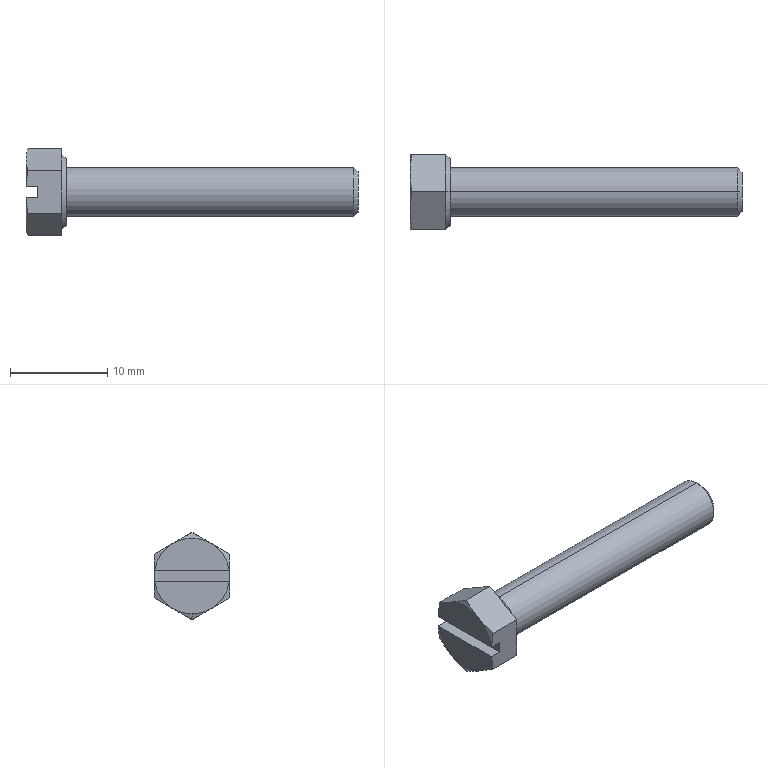Part | SolidWorks | features RevCut 2, Boss 1, Chamfer 1, Cut 1, Extrusion 1, Fillet 1, LPattern 1, Revolution 1 | 1 solid | 32 faces | box 34.15 x 7.78 x 8.984 mm | volume 788.587 mm3 | plane 19 | cone 11 | cylinder 2 | commonest cylinder face diameters 5 x2
STEP:
#1=CARTESIAN_POINT('',(0.,-1.945,-3.369));
#2=VERTEX_POINT('',#1);
#3=CARTESIAN_POINT('',(0.,0.,-3.89));
#4=VERTEX_POINT('',#3);
#5=CARTESIAN_POINT('',(0.,0.,0.));
#6=DIRECTION('',(1.,0.,0.));
#7=DIRECTION('',(0.,0.,-1.));
#8=AXIS2_PLACEMENT_3D('',#5,#6,#7);
#9=CIRCLE('',#8,3.89);
#10=EDGE_CURVE('',#2,#4,#9,.T.);
#11=ORIENTED_EDGE('',*,*,#10,.T.);
#12=CARTESIAN_POINT('',(0.219,0.,-4.492));
#13=VERTEX_POINT('',#12);
#14=CARTESIAN_POINT('',(0.,0.,-3.89));
#15=DIRECTION('',(0.342,0.,-0.9397));
#16=VECTOR('',#15,1000.);
#17=LINE('',#14,#16);
#18=EDGE_CURVE('',#4,#13,#17,.T.);
#19=ORIENTED_EDGE('',*,*,#18,.T.);
#20=CARTESIAN_POINT('',(0.219,0.,-4.492));
#21=CARTESIAN_POINT('',(0.08279,-0.6483,-4.117));
#22=CARTESIAN_POINT('',(0.,-1.297,-3.743));
#23=CARTESIAN_POINT('',(0.,-1.945,-3.369));
#24=B_SPLINE_CURVE_WITH_KNOTS('',3,(#20,#21,#22,#23),.UNSPECIFIED.,.F.,.F.,(4,4),(0.000000231,0.002246),.UNSPECIFIED.);
#25=EDGE_CURVE('',#13,#2,#24,.T.);
#26=ORIENTED_EDGE('',*,*,#25,.T.);
#27=EDGE_LOOP('',(#11,#19,#26));
#28=FACE_OUTER_BOUND('',#27,.T.);
#29=CARTESIAN_POINT('',(0.,0.,0.));
#30=DIRECTION('',(1.,0.,0.));
#31=DIRECTION('',(0.,0.,-1.));
#32=AXIS2_PLACEMENT_3D('',#29,#30,#31);
#33=CONICAL_SURFACE('',#32,3.89,1.222);
#34=ADVANCED_FACE('',(#28),#33,.T.);
#35=CARTESIAN_POINT('',(34.15,0.,-2.067));
#36=VERTEX_POINT('',#35);
#37=CARTESIAN_POINT('',(34.15,0.,2.067));
#38=VERTEX_POINT('',#37);
#39=CARTESIAN_POINT('',(34.15,0.,0.));
#40=DIRECTION('',(1.,0.,0.));
#41=DIRECTION('',(0.,0.,-1.));
#42=AXIS2_PLACEMENT_3D('',#39,#40,#41);
#43=CIRCLE('',#42,2.067);
#44=EDGE_CURVE('',#36,#38,#43,.T.);
#45=ORIENTED_EDGE('',*,*,#44,.F.);
#46=CARTESIAN_POINT('',(33.717,0.,-2.5));
#47=VERTEX_POINT('',#46);
#48=CARTESIAN_POINT('',(34.15,0.,-2.067));
#49=DIRECTION('',(-0.7071,0.,-0.7071));
#50=VECTOR('',#49,1000.);
#51=LINE('',#48,#50);
#52=EDGE_CURVE('',#36,#47,#51,.T.);
#53=ORIENTED_EDGE('',*,*,#52,.T.);
#54=CARTESIAN_POINT('',(33.717,0.,2.5));
#55=VERTEX_POINT('',#54);
#56=CARTESIAN_POINT('',(33.717,0.,0.));
#57=DIRECTION('',(-1.,0.,0.));
#58=DIRECTION('',(0.,0.,-1.));
#59=AXIS2_PLACEMENT_3D('',#56,#57,#58);
#60=CIRCLE('',#59,2.5);
#61=EDGE_CURVE('',#55,#47,#60,.T.);
#62=ORIENTED_EDGE('',*,*,#61,.F.);
#63=CARTESIAN_POINT('',(34.15,0.,2.067));
#64=DIRECTION('',(-0.7071,0.,0.7071));
#65=VECTOR('',#64,1000.);
#66=LINE('',#63,#65);
#67=EDGE_CURVE('',#38,#55,#66,.T.);
#68=ORIENTED_EDGE('',*,*,#67,.F.);
#69=EDGE_LOOP('',(#45,#53,#62,#68));
#70=FACE_OUTER_BOUND('',#69,.T.);
#71=CARTESIAN_POINT('',(34.15,0.,0.));
#72=DIRECTION('',(-1.,0.,0.));
#73=DIRECTION('',(0.,0.,1.));
#74=AXIS2_PLACEMENT_3D('',#71,#72,#73);
#75=CONICAL_SURFACE('',#74,2.067,0.7854);
#76=ADVANCED_FACE('',(#70),#75,.T.);
#77=ORIENTED_EDGE('',*,*,#61,.T.);
#78=CARTESIAN_POINT('',(4.15,0.,-2.5));
#79=VERTEX_POINT('',#78);
#80=CARTESIAN_POINT('',(34.15,0.,-2.5));
#81=DIRECTION('',(-1.,0.,0.));
#82=VECTOR('',#81,1000.);
#83=LINE('',#80,#82);
#84=EDGE_CURVE('',#47,#79,#83,.T.);
#85=ORIENTED_EDGE('',*,*,#84,.T.);
#86=CARTESIAN_POINT('',(4.15,0.,2.5));
#87=VERTEX_POINT('',#86);
#88=CARTESIAN_POINT('',(4.15,0.,0.));
#89=DIRECTION('',(1.,0.,0.));
#90=DIRECTION('',(0.,0.,-1.));
#91=AXIS2_PLACEMENT_3D('',#88,#89,#90);
#92=CIRCLE('',#91,2.5);
#93=EDGE_CURVE('',#79,#87,#92,.T.);
#94=ORIENTED_EDGE('',*,*,#93,.T.);
#95=CARTESIAN_POINT('',(34.15,0.,2.5));
#96=DIRECTION('',(-1.,0.,0.));
#97=VECTOR('',#96,1000.);
#98=LINE('',#95,#97);
#99=EDGE_CURVE('',#55,#87,#98,.T.);
#100=ORIENTED_EDGE('',*,*,#99,.F.);
#101=EDGE_LOOP('',(#77,#85,#94,#100));
#102=FACE_OUTER_BOUND('',#101,.T.);
#103=CARTESIAN_POINT('',(34.15,0.,0.));
#104=DIRECTION('',(-1.,0.,0.));
#105=DIRECTION('',(0.,0.,1.));
#106=AXIS2_PLACEMENT_3D('',#103,#104,#105);
#107=CYLINDRICAL_SURFACE('',#106,2.5);
#108=ADVANCED_FACE('',(#102),#107,.T.);
#109=CARTESIAN_POINT('',(4.15,0.,3.44));
#110=VERTEX_POINT('',#109);
#111=CARTESIAN_POINT('',(4.15,0.,-3.44));
#112=VERTEX_POINT('',#111);
#113=CARTESIAN_POINT('',(4.15,0.,0.));
#114=DIRECTION('',(-1.,0.,0.));
#115=DIRECTION('',(0.,0.,1.));
#116=AXIS2_PLACEMENT_3D('',#113,#114,#115);
#117=CIRCLE('',#116,3.44);
#118=EDGE_CURVE('',#110,#112,#117,.T.);
#119=ORIENTED_EDGE('',*,*,#118,.T.);
#120=CARTESIAN_POINT('',(3.65,0.,-3.89));
#121=VERTEX_POINT('',#120);
#122=CARTESIAN_POINT('',(3.65,0.,-3.89));
#123=DIRECTION('',(-0.7433,0.,-0.669));
#124=VECTOR('',#123,1000.);
#125=LINE('',#122,#124);
#126=EDGE_CURVE('',#112,#121,#125,.T.);
#127=ORIENTED_EDGE('',*,*,#126,.T.);
#128=CARTESIAN_POINT('',(3.65,1.945,-3.369));
#129=VERTEX_POINT('',#128);
#130=CARTESIAN_POINT('',(3.65,0.,0.));
#131=DIRECTION('',(-1.,0.,0.));
#132=DIRECTION('',(0.,0.,1.));
#133=AXIS2_PLACEMENT_3D('',#130,#131,#132);
#134=CIRCLE('',#133,3.89);
#135=EDGE_CURVE('',#129,#121,#134,.T.);
#136=ORIENTED_EDGE('',*,*,#135,.F.);
#137=CARTESIAN_POINT('',(3.65,3.89,0.));
#138=VERTEX_POINT('',#137);
#139=CARTESIAN_POINT('',(3.65,0.,0.));
#140=DIRECTION('',(-1.,0.,0.));
#141=DIRECTION('',(0.,0.,1.));
#142=AXIS2_PLACEMENT_3D('',#139,#140,#141);
#143=CIRCLE('',#142,3.89);
#144=EDGE_CURVE('',#138,#129,#143,.T.);
#145=ORIENTED_EDGE('',*,*,#144,.F.);
#146=CARTESIAN_POINT('',(3.65,1.945,3.369));
#147=VERTEX_POINT('',#146);
#148=CARTESIAN_POINT('',(3.65,0.,0.));
#149=DIRECTION('',(-1.,0.,0.));
#150=DIRECTION('',(0.,0.,1.));
#151=AXIS2_PLACEMENT_3D('',#148,#149,#150);
#152=CIRCLE('',#151,3.89);
#153=EDGE_CURVE('',#147,#138,#152,.T.);
#154=ORIENTED_EDGE('',*,*,#153,.F.);
#155=CARTESIAN_POINT('',(3.65,0.,3.89));
#156=VERTEX_POINT('',#155);
#157=CARTESIAN_POINT('',(3.65,0.,0.));
#158=DIRECTION('',(-1.,0.,0.));
#159=DIRECTION('',(0.,0.,1.));
#160=AXIS2_PLACEMENT_3D('',#157,#158,#159);
#161=CIRCLE('',#160,3.89);
#162=EDGE_CURVE('',#156,#147,#161,.T.);
#163=ORIENTED_EDGE('',*,*,#162,.F.);
#164=CARTESIAN_POINT('',(3.65,0.,3.89));
#165=DIRECTION('',(-0.7433,0.,0.669));
#166=VECTOR('',#165,1000.);
#167=LINE('',#164,#166);
#168=EDGE_CURVE('',#110,#156,#167,.T.);
#169=ORIENTED_EDGE('',*,*,#168,.F.);
#170=EDGE_LOOP('',(#119,#127,#136,#145,#154,#163,#169));
#171=FACE_OUTER_BOUND('',#170,.T.);
#172=CARTESIAN_POINT('',(3.65,0.,0.));
#173=DIRECTION('',(-1.,0.,0.));
#174=DIRECTION('',(0.,0.,1.));
#175=AXIS2_PLACEMENT_3D('',#172,#173,#174);
#176=CONICAL_SURFACE('',#175,3.89,0.7328);
#177=ADVANCED_FACE('',(#171),#176,.T.);
#178=CARTESIAN_POINT('',(0.,-3.843,-0.6));
#179=VERTEX_POINT('',#178);
#180=CARTESIAN_POINT('',(0.,0.,0.));
#181=DIRECTION('',(1.,0.,0.));
#182=DIRECTION('',(0.,0.,-1.));
#183=AXIS2_PLACEMENT_3D('',#180,#181,#182);
#184=CIRCLE('',#183,3.89);
#185=EDGE_CURVE('',#179,#2,#184,.T.);
#186=ORIENTED_EDGE('',*,*,#185,.F.);
#187=CARTESIAN_POINT('',(0.,3.843,-0.6));
#188=VERTEX_POINT('',#187);
#189=CARTESIAN_POINT('',(0.,-3.89,-0.6));
#190=DIRECTION('',(0.,1.,0.));
#191=VECTOR('',#190,1000.);
#192=LINE('',#189,#191);
#193=EDGE_CURVE('',#179,#188,#192,.T.);
#194=ORIENTED_EDGE('',*,*,#193,.T.);
#195=CARTESIAN_POINT('',(0.,1.945,-3.369));
#196=VERTEX_POINT('',#195);
#197=CARTESIAN_POINT('',(0.,0.,0.));
#198=DIRECTION('',(1.,0.,0.));
#199=DIRECTION('',(0.,0.,-1.));
#200=AXIS2_PLACEMENT_3D('',#197,#198,#199);
#201=CIRCLE('',#200,3.89);
#202=EDGE_CURVE('',#196,#188,#201,.T.);
#203=ORIENTED_EDGE('',*,*,#202,.F.);
#204=CARTESIAN_POINT('',(0.,0.,0.));
#205=DIRECTION('',(1.,0.,0.));
#206=DIRECTION('',(0.,0.,-1.));
#207=AXIS2_PLACEMENT_3D('',#204,#205,#206);
#208=CIRCLE('',#207,3.89);
#209=EDGE_CURVE('',#4,#196,#208,.T.);
#210=ORIENTED_EDGE('',*,*,#209,.F.);
#211=ORIENTED_EDGE('',*,*,#10,.F.);
#212=EDGE_LOOP('',(#186,#194,#203,#210,#211));
#213=FACE_OUTER_BOUND('',#212,.T.);
#214=CARTESIAN_POINT('',(0.,-3.89,-2.246));
#215=DIRECTION('',(1.,0.,0.));
#216=DIRECTION('',(0.,0.,-1.));
#217=AXIS2_PLACEMENT_3D('',#214,#215,#216);
#218=PLANE('',#217);
#219=ADVANCED_FACE('',(#213),#218,.F.);
#220=CARTESIAN_POINT('',(1.2,-3.89,0.6));
#221=VERTEX_POINT('',#220);
#222=CARTESIAN_POINT('',(1.2,-3.89,-0.6));
#223=VERTEX_POINT('',#222);
#224=CARTESIAN_POINT('',(1.2,-3.89,0.6));
#225=DIRECTION('',(0.,0.,-1.));
#226=VECTOR('',#225,1000.);
#227=LINE('',#224,#226);
#228=EDGE_CURVE('',#221,#223,#227,.T.);
#229=ORIENTED_EDGE('',*,*,#228,.T.);
#230=CARTESIAN_POINT('',(0.01674,-3.89,-0.6));
#231=VERTEX_POINT('',#230);
#232=CARTESIAN_POINT('',(1.2,-3.89,-0.6));
#233=DIRECTION('',(-1.,0.,0.));
#234=VECTOR('',#233,1000.);
#235=LINE('',#232,#234);
#236=EDGE_CURVE('',#223,#231,#235,.T.);
#237=ORIENTED_EDGE('',*,*,#236,.T.);
#238=CARTESIAN_POINT('',(0.219,-3.89,-2.246));
#239=VERTEX_POINT('',#238);
#240=CARTESIAN_POINT('',(0.219,-3.89,-2.246));
#241=CARTESIAN_POINT('',(0.1199,-3.89,-1.701));
#242=CARTESIAN_POINT('',(0.04719,-3.89,-1.149));
#243=CARTESIAN_POINT('',(0.01674,-3.89,-0.6));
#244=B_SPLINE_CURVE_WITH_KNOTS('',3,(#240,#241,#242,#243),.UNSPECIFIED.,.F.,.F.,(4,4),(0.003821,0.005479),.UNSPECIFIED.);
#245=EDGE_CURVE('',#239,#231,#244,.T.);
#246=ORIENTED_EDGE('',*,*,#245,.F.);
#247=CARTESIAN_POINT('',(3.65,-3.89,-2.246));
#248=VERTEX_POINT('',#247);
#249=CARTESIAN_POINT('',(3.65,-3.89,-2.246));
#250=DIRECTION('',(-1.,0.,0.));
#251=VECTOR('',#250,1000.);
#252=LINE('',#249,#251);
#253=EDGE_CURVE('',#248,#239,#252,.T.);
#254=ORIENTED_EDGE('',*,*,#253,.F.);
#255=CARTESIAN_POINT('',(3.65,-3.89,0.));
#256=VERTEX_POINT('',#255);
#257=CARTESIAN_POINT('',(3.65,-3.89,2.246));
#258=DIRECTION('',(0.,0.,-1.));
#259=VECTOR('',#258,1000.);
#260=LINE('',#257,#259);
#261=EDGE_CURVE('',#256,#248,#260,.T.);
#262=ORIENTED_EDGE('',*,*,#261,.F.);
#263=CARTESIAN_POINT('',(3.65,-3.89,2.246));
#264=VERTEX_POINT('',#263);
#265=CARTESIAN_POINT('',(3.65,-3.89,2.246));
#266=DIRECTION('',(0.,0.,-1.));
#267=VECTOR('',#266,1000.);
#268=LINE('',#265,#267);
#269=EDGE_CURVE('',#264,#256,#268,.T.);
#270=ORIENTED_EDGE('',*,*,#269,.F.);
#271=CARTESIAN_POINT('',(0.219,-3.89,2.246));
#272=VERTEX_POINT('',#271);
#273=CARTESIAN_POINT('',(3.65,-3.89,2.246));
#274=DIRECTION('',(-1.,0.,0.));
#275=VECTOR('',#274,1000.);
#276=LINE('',#273,#275);
#277=EDGE_CURVE('',#264,#272,#276,.T.);
#278=ORIENTED_EDGE('',*,*,#277,.T.);
#279=CARTESIAN_POINT('',(0.01674,-3.89,0.6));
#280=VERTEX_POINT('',#279);
#281=CARTESIAN_POINT('',(0.01674,-3.89,0.6));
#282=CARTESIAN_POINT('',(0.04723,-3.89,1.149));
#283=CARTESIAN_POINT('',(0.1194,-3.89,1.698));
#284=CARTESIAN_POINT('',(0.219,-3.89,2.246));
#285=B_SPLINE_CURVE_WITH_KNOTS('',3,(#281,#282,#283,#284),.UNSPECIFIED.,.F.,.F.,(4,4),(0.00669,0.008354),.UNSPECIFIED.);
#286=EDGE_CURVE('',#280,#272,#285,.T.);
#287=ORIENTED_EDGE('',*,*,#286,.F.);
#288=CARTESIAN_POINT('',(0.,-3.89,0.6));
#289=DIRECTION('',(1.,0.,0.));
#290=VECTOR('',#289,1000.);
#291=LINE('',#288,#290);
#292=EDGE_CURVE('',#280,#221,#291,.T.);
#293=ORIENTED_EDGE('',*,*,#292,.T.);
#294=EDGE_LOOP('',(#229,#237,#246,#254,#262,#270,#278,#287,#293));
#295=FACE_OUTER_BOUND('',#294,.T.);
#296=CARTESIAN_POINT('',(3.65,-3.89,2.246));
#297=DIRECTION('',(0.,1.,0.));
#298=DIRECTION('',(0.,0.,1.));
#299=AXIS2_PLACEMENT_3D('',#296,#297,#298);
#300=PLANE('',#299);
#301=ADVANCED_FACE('',(#295),#300,.F.);
#302=ORIENTED_EDGE('',*,*,#25,.F.);
#303=CARTESIAN_POINT('',(3.65,0.,-4.492));
#304=VERTEX_POINT('',#303);
#305=CARTESIAN_POINT('',(3.65,0.,-4.492));
#306=DIRECTION('',(-1.,0.,0.));
#307=VECTOR('',#306,1000.);
#308=LINE('',#305,#307);
#309=EDGE_CURVE('',#304,#13,#308,.T.);
#310=ORIENTED_EDGE('',*,*,#309,.F.);
#311=CARTESIAN_POINT('',(3.65,-1.945,-3.369));
#312=VERTEX_POINT('',#311);
#313=CARTESIAN_POINT('',(3.65,-3.89,-2.246));
#314=DIRECTION('',(0.,0.866,-0.5));
#315=VECTOR('',#314,1000.);
#316=LINE('',#313,#315);
#317=EDGE_CURVE('',#312,#304,#316,.T.);
#318=ORIENTED_EDGE('',*,*,#317,.F.);
#319=CARTESIAN_POINT('',(3.65,-3.89,-2.246));
#320=DIRECTION('',(0.,0.866,-0.5));
#321=VECTOR('',#320,1000.);
#322=LINE('',#319,#321);
#323=EDGE_CURVE('',#248,#312,#322,.T.);
#324=ORIENTED_EDGE('',*,*,#323,.F.);
#325=ORIENTED_EDGE('',*,*,#253,.T.);
#326=CARTESIAN_POINT('',(0.,-1.945,-3.369));
#327=CARTESIAN_POINT('',(0.,-2.593,-2.995));
#328=CARTESIAN_POINT('',(0.08279,-3.242,-2.62));
#329=CARTESIAN_POINT('',(0.219,-3.89,-2.246));
#330=B_SPLINE_CURVE_WITH_KNOTS('',3,(#326,#327,#328,#329),.UNSPECIFIED.,.F.,.F.,(4,4),(0.002246,0.004492),.UNSPECIFIED.);
#331=EDGE_CURVE('',#2,#239,#330,.T.);
#332=ORIENTED_EDGE('',*,*,#331,.F.);
#333=EDGE_LOOP('',(#302,#310,#318,#324,#325,#332));
#334=FACE_OUTER_BOUND('',#333,.T.);
#335=CARTESIAN_POINT('',(3.65,-3.89,-2.246));
#336=DIRECTION('',(0.,0.5,0.866));
#337=DIRECTION('',(0.,-0.866,0.5));
#338=AXIS2_PLACEMENT_3D('',#335,#336,#337);
#339=PLANE('',#338);
#340=ADVANCED_FACE('',(#334),#339,.F.);
#341=CARTESIAN_POINT('',(0.219,3.89,-2.246));
#342=VERTEX_POINT('',#341);
#343=CARTESIAN_POINT('',(0.219,3.89,-2.246));
#344=CARTESIAN_POINT('',(0.08279,3.242,-2.62));
#345=CARTESIAN_POINT('',(0.,2.593,-2.995));
#346=CARTESIAN_POINT('',(0.,1.945,-3.369));
#347=B_SPLINE_CURVE_WITH_KNOTS('',3,(#343,#344,#345,#346),.UNSPECIFIED.,.F.,.F.,(4,4),(0.000000231,0.002246),.UNSPECIFIED.);
#348=EDGE_CURVE('',#342,#196,#347,.T.);
#349=ORIENTED_EDGE('',*,*,#348,.F.);
#350=CARTESIAN_POINT('',(3.65,3.89,-2.246));
#351=VERTEX_POINT('',#350);
#352=CARTESIAN_POINT('',(3.65,3.89,-2.246));
#353=DIRECTION('',(-1.,0.,0.));
#354=VECTOR('',#353,1000.);
#355=LINE('',#352,#354);
#356=EDGE_CURVE('',#351,#342,#355,.T.);
#357=ORIENTED_EDGE('',*,*,#356,.F.);
#358=CARTESIAN_POINT('',(3.65,0.,-4.492));
#359=DIRECTION('',(0.,0.866,0.5));
#360=VECTOR('',#359,1000.);
#361=LINE('',#358,#360);
#362=EDGE_CURVE('',#129,#351,#361,.T.);
#363=ORIENTED_EDGE('',*,*,#362,.F.);
#364=CARTESIAN_POINT('',(3.65,0.,-4.492));
#365=DIRECTION('',(0.,0.866,0.5));
#366=VECTOR('',#365,1000.);
#367=LINE('',#364,#366);
#368=EDGE_CURVE('',#304,#129,#367,.T.);
#369=ORIENTED_EDGE('',*,*,#368,.F.);
#370=ORIENTED_EDGE('',*,*,#309,.T.);
#371=CARTESIAN_POINT('',(0.,1.945,-3.369));
#372=CARTESIAN_POINT('',(0.,1.297,-3.743));
#373=CARTESIAN_POINT('',(0.08279,0.6483,-4.117));
#374=CARTESIAN_POINT('',(0.219,0.,-4.492));
#375=B_SPLINE_CURVE_WITH_KNOTS('',3,(#371,#372,#373,#374),.UNSPECIFIED.,.F.,.F.,(4,4),(0.002246,0.004492),.UNSPECIFIED.);
#376=EDGE_CURVE('',#196,#13,#375,.T.);
#377=ORIENTED_EDGE('',*,*,#376,.F.);
#378=EDGE_LOOP('',(#349,#357,#363,#369,#370,#377));
#379=FACE_OUTER_BOUND('',#378,.T.);
#380=CARTESIAN_POINT('',(3.65,0.,-4.492));
#381=DIRECTION('',(0.,-0.5,0.866));
#382=DIRECTION('',(0.,-0.866,-0.5));
#383=AXIS2_PLACEMENT_3D('',#380,#381,#382);
#384=PLANE('',#383);
#385=ADVANCED_FACE('',(#379),#384,.F.);
#386=CARTESIAN_POINT('',(0.01674,3.89,-0.6));
#387=VERTEX_POINT('',#386);
#388=CARTESIAN_POINT('',(0.01674,3.89,-0.6));
#389=CARTESIAN_POINT('',(0.04719,3.89,-1.149));
#390=CARTESIAN_POINT('',(0.1199,3.89,-1.701));
#391=CARTESIAN_POINT('',(0.219,3.89,-2.246));
#392=B_SPLINE_CURVE_WITH_KNOTS('',3,(#388,#389,#390,#391),.UNSPECIFIED.,.F.,.F.,(4,4),(0.01097,0.01262),.UNSPECIFIED.);
#393=EDGE_CURVE('',#387,#342,#392,.T.);
#394=ORIENTED_EDGE('',*,*,#393,.F.);
#395=CARTESIAN_POINT('',(1.2,3.89,-0.6));
#396=VERTEX_POINT('',#395);
#397=CARTESIAN_POINT('',(1.2,3.89,-0.6));
#398=DIRECTION('',(-1.,0.,0.));
#399=VECTOR('',#398,1000.);
#400=LINE('',#397,#399);
#401=EDGE_CURVE('',#396,#387,#400,.T.);
#402=ORIENTED_EDGE('',*,*,#401,.F.);
#403=CARTESIAN_POINT('',(1.2,3.89,0.6));
#404=VERTEX_POINT('',#403);
#405=CARTESIAN_POINT('',(1.2,3.89,0.6));
#406=DIRECTION('',(0.,0.,-1.));
#407=VECTOR('',#406,1000.);
#408=LINE('',#405,#407);
#409=EDGE_CURVE('',#404,#396,#408,.T.);
#410=ORIENTED_EDGE('',*,*,#409,.F.);
#411=CARTESIAN_POINT('',(0.01674,3.89,0.6));
#412=VERTEX_POINT('',#411);
#413=CARTESIAN_POINT('',(0.,3.89,0.6));
#414=DIRECTION('',(1.,0.,0.));
#415=VECTOR('',#414,1000.);
#416=LINE('',#413,#415);
#417=EDGE_CURVE('',#412,#404,#416,.T.);
#418=ORIENTED_EDGE('',*,*,#417,.F.);
#419=CARTESIAN_POINT('',(0.219,3.89,2.246));
#420=VERTEX_POINT('',#419);
#421=CARTESIAN_POINT('',(0.219,3.89,2.246));
#422=CARTESIAN_POINT('',(0.1194,3.89,1.698));
#423=CARTESIAN_POINT('',(0.04723,3.89,1.149));
#424=CARTESIAN_POINT('',(0.01674,3.89,0.6));
#425=B_SPLINE_CURVE_WITH_KNOTS('',3,(#421,#422,#423,#424),.UNSPECIFIED.,.F.,.F.,(4,4),(0.008099,0.009759),.UNSPECIFIED.);
#426=EDGE_CURVE('',#420,#412,#425,.T.);
#427=ORIENTED_EDGE('',*,*,#426,.F.);
#428=CARTESIAN_POINT('',(3.65,3.89,2.246));
#429=VERTEX_POINT('',#428);
#430=CARTESIAN_POINT('',(3.65,3.89,2.246));
#431=DIRECTION('',(-1.,0.,0.));
#432=VECTOR('',#431,1000.);
#433=LINE('',#430,#432);
#434=EDGE_CURVE('',#429,#420,#433,.T.);
#435=ORIENTED_EDGE('',*,*,#434,.F.);
#436=CARTESIAN_POINT('',(3.65,3.89,-2.246));
#437=DIRECTION('',(0.,0.,1.));
#438=VECTOR('',#437,1000.);
#439=LINE('',#436,#438);
#440=EDGE_CURVE('',#138,#429,#439,.T.);
#441=ORIENTED_EDGE('',*,*,#440,.F.);
#442=CARTESIAN_POINT('',(3.65,3.89,-2.246));
#443=DIRECTION('',(0.,0.,1.));
#444=VECTOR('',#443,1000.);
#445=LINE('',#442,#444);
#446=EDGE_CURVE('',#351,#138,#445,.T.);
#447=ORIENTED_EDGE('',*,*,#446,.F.);
#448=ORIENTED_EDGE('',*,*,#356,.T.);
#449=EDGE_LOOP('',(#394,#402,#410,#418,#427,#435,#441,#447,#448));
#450=FACE_OUTER_BOUND('',#449,.T.);
#451=CARTESIAN_POINT('',(3.65,3.89,-2.246));
#452=DIRECTION('',(0.,-1.,0.));
#453=DIRECTION('',(0.,0.,-1.));
#454=AXIS2_PLACEMENT_3D('',#451,#452,#453);
#455=PLANE('',#454);
#456=ADVANCED_FACE('',(#450),#455,.F.);
#457=CARTESIAN_POINT('',(0.219,0.,4.492));
#458=VERTEX_POINT('',#457);
#459=CARTESIAN_POINT('',(0.,1.945,3.369));
#460=VERTEX_POINT('',#459);
#461=CARTESIAN_POINT('',(0.219,0.,4.492));
#462=CARTESIAN_POINT('',(0.08279,0.6483,4.117));
#463=CARTESIAN_POINT('',(0.,1.297,3.743));
#464=CARTESIAN_POINT('',(0.,1.945,3.369));
#465=B_SPLINE_CURVE_WITH_KNOTS('',3,(#461,#462,#463,#464),.UNSPECIFIED.,.F.,.F.,(4,4),(0.000000231,0.002246),.UNSPECIFIED.);
#466=EDGE_CURVE('',#458,#460,#465,.T.);
#467=ORIENTED_EDGE('',*,*,#466,.F.);
#468=CARTESIAN_POINT('',(3.65,0.,4.492));
#469=VERTEX_POINT('',#468);
#470=CARTESIAN_POINT('',(3.65,0.,4.492));
#471=DIRECTION('',(-1.,0.,0.));
#472=VECTOR('',#471,1000.);
#473=LINE('',#470,#472);
#474=EDGE_CURVE('',#469,#458,#473,.T.);
#475=ORIENTED_EDGE('',*,*,#474,.F.);
#476=CARTESIAN_POINT('',(3.65,3.89,2.246));
#477=DIRECTION('',(0.,-0.866,0.5));
#478=VECTOR('',#477,1000.);
#479=LINE('',#476,#478);
#480=EDGE_CURVE('',#147,#469,#479,.T.);
#481=ORIENTED_EDGE('',*,*,#480,.F.);
#482=CARTESIAN_POINT('',(3.65,3.89,2.246));
#483=DIRECTION('',(0.,-0.866,0.5));
#484=VECTOR('',#483,1000.);
#485=LINE('',#482,#484);
#486=EDGE_CURVE('',#429,#147,#485,.T.);
#487=ORIENTED_EDGE('',*,*,#486,.F.);
#488=ORIENTED_EDGE('',*,*,#434,.T.);
#489=CARTESIAN_POINT('',(0.,1.945,3.369));
#490=CARTESIAN_POINT('',(0.,2.593,2.995));
#491=CARTESIAN_POINT('',(0.08279,3.242,2.62));
#492=CARTESIAN_POINT('',(0.219,3.89,2.246));
#493=B_SPLINE_CURVE_WITH_KNOTS('',3,(#489,#490,#491,#492),.UNSPECIFIED.,.F.,.F.,(4,4),(0.002246,0.004492),.UNSPECIFIED.);
#494=EDGE_CURVE('',#460,#420,#493,.T.);
#495=ORIENTED_EDGE('',*,*,#494,.F.);
#496=EDGE_LOOP('',(#467,#475,#481,#487,#488,#495));
#497=FACE_OUTER_BOUND('',#496,.T.);
#498=CARTESIAN_POINT('',(3.65,3.89,2.246));
#499=DIRECTION('',(0.,-0.5,-0.866));
#500=DIRECTION('',(0.,0.866,-0.5));
#501=AXIS2_PLACEMENT_3D('',#498,#499,#500);
#502=PLANE('',#501);
#503=ADVANCED_FACE('',(#497),#502,.F.);
#504=CARTESIAN_POINT('',(0.,-1.945,3.369));
#505=VERTEX_POINT('',#504);
#506=CARTESIAN_POINT('',(0.219,-3.89,2.246));
#507=CARTESIAN_POINT('',(0.08279,-3.242,2.62));
#508=CARTESIAN_POINT('',(0.,-2.593,2.995));
#509=CARTESIAN_POINT('',(0.,-1.945,3.369));
#510=B_SPLINE_CURVE_WITH_KNOTS('',3,(#506,#507,#508,#509),.UNSPECIFIED.,.F.,.F.,(4,4),(0.000000231,0.002246),.UNSPECIFIED.);
#511=EDGE_CURVE('',#272,#505,#510,.T.);
#512=ORIENTED_EDGE('',*,*,#511,.F.);
#513=ORIENTED_EDGE('',*,*,#277,.F.);
#514=CARTESIAN_POINT('',(3.65,-1.945,3.369));
#515=VERTEX_POINT('',#514);
#516=CARTESIAN_POINT('',(3.65,0.,4.492));
#517=DIRECTION('',(0.,-0.866,-0.5));
#518=VECTOR('',#517,1000.);
#519=LINE('',#516,#518);
#520=EDGE_CURVE('',#515,#264,#519,.T.);
#521=ORIENTED_EDGE('',*,*,#520,.F.);
#522=CARTESIAN_POINT('',(3.65,0.,4.492));
#523=DIRECTION('',(0.,-0.866,-0.5));
#524=VECTOR('',#523,1000.);
#525=LINE('',#522,#524);
#526=EDGE_CURVE('',#469,#515,#525,.T.);
#527=ORIENTED_EDGE('',*,*,#526,.F.);
#528=ORIENTED_EDGE('',*,*,#474,.T.);
#529=CARTESIAN_POINT('',(0.,-1.945,3.369));
#530=CARTESIAN_POINT('',(0.,-1.297,3.743));
#531=CARTESIAN_POINT('',(0.08279,-0.6483,4.117));
#532=CARTESIAN_POINT('',(0.219,0.,4.492));
#533=B_SPLINE_CURVE_WITH_KNOTS('',3,(#529,#530,#531,#532),.UNSPECIFIED.,.F.,.F.,(4,4),(0.002246,0.004492),.UNSPECIFIED.);
#534=EDGE_CURVE('',#505,#458,#533,.T.);
#535=ORIENTED_EDGE('',*,*,#534,.F.);
#536=EDGE_LOOP('',(#512,#513,#521,#527,#528,#535));
#537=FACE_OUTER_BOUND('',#536,.T.);
#538=CARTESIAN_POINT('',(3.65,0.,4.492));
#539=DIRECTION('',(0.,0.5,-0.866));
#540=DIRECTION('',(0.,0.866,0.5));
#541=AXIS2_PLACEMENT_3D('',#538,#539,#540);
#542=PLANE('',#541);
#543=ADVANCED_FACE('',(#537),#542,.F.);
#544=ORIENTED_EDGE('',*,*,#118,.F.);
#545=CARTESIAN_POINT('',(4.15,0.,0.));
#546=DIRECTION('',(-1.,0.,0.));
#547=DIRECTION('',(0.,0.,1.));
#548=AXIS2_PLACEMENT_3D('',#545,#546,#547);
#549=CIRCLE('',#548,3.44);
#550=EDGE_CURVE('',#112,#110,#549,.T.);
#551=ORIENTED_EDGE('',*,*,#550,.F.);
#552=EDGE_LOOP('',(#544,#551));
#553=FACE_OUTER_BOUND('',#552,.T.);
#554=CARTESIAN_POINT('',(4.15,0.,0.));
#555=DIRECTION('',(1.,0.,0.));
#556=DIRECTION('',(0.,0.,-1.));
#557=AXIS2_PLACEMENT_3D('',#554,#555,#556);
#558=CIRCLE('',#557,2.5);
#559=EDGE_CURVE('',#87,#79,#558,.T.);
#560=ORIENTED_EDGE('',*,*,#559,.F.);
#561=ORIENTED_EDGE('',*,*,#93,.F.);
#562=EDGE_LOOP('',(#560,#561));
#563=FACE_BOUND('',#562,.T.);
#564=CARTESIAN_POINT('',(4.15,0.,0.));
#565=DIRECTION('',(1.,0.,0.));
#566=DIRECTION('',(0.,0.,-1.));
#567=AXIS2_PLACEMENT_3D('',#564,#565,#566);
#568=PLANE('',#567);
#569=ADVANCED_FACE('',(#553,#563),#568,.T.);
#570=ORIENTED_EDGE('',*,*,#486,.T.);
#571=ORIENTED_EDGE('',*,*,#153,.T.);
#572=ORIENTED_EDGE('',*,*,#440,.T.);
#573=EDGE_LOOP('',(#570,#571,#572));
#574=FACE_OUTER_BOUND('',#573,.T.);
#575=CARTESIAN_POINT('',(3.65,-3.89,-2.246));
#576=DIRECTION('',(1.,0.,0.));
#577=DIRECTION('',(0.,0.,-1.));
#578=AXIS2_PLACEMENT_3D('',#575,#576,#577);
#579=PLANE('',#578);
#580=ADVANCED_FACE('',(#574),#579,.T.);
#581=ORIENTED_EDGE('',*,*,#446,.T.);
#582=ORIENTED_EDGE('',*,*,#144,.T.);
#583=ORIENTED_EDGE('',*,*,#362,.T.);
#584=EDGE_LOOP('',(#581,#582,#583));
#585=FACE_OUTER_BOUND('',#584,.T.);
#586=CARTESIAN_POINT('',(3.65,-3.89,-2.246));
#587=DIRECTION('',(1.,0.,0.));
#588=DIRECTION('',(0.,0.,-1.));
#589=AXIS2_PLACEMENT_3D('',#586,#587,#588);
#590=PLANE('',#589);
#591=ADVANCED_FACE('',(#585),#590,.T.);
#592=ORIENTED_EDGE('',*,*,#368,.T.);
#593=ORIENTED_EDGE('',*,*,#135,.T.);
#594=CARTESIAN_POINT('',(3.65,0.,0.));
#595=DIRECTION('',(-1.,0.,0.));
#596=DIRECTION('',(0.,0.,1.));
#597=AXIS2_PLACEMENT_3D('',#594,#595,#596);
#598=CIRCLE('',#597,3.89);
#599=EDGE_CURVE('',#121,#312,#598,.T.);
#600=ORIENTED_EDGE('',*,*,#599,.T.);
#601=ORIENTED_EDGE('',*,*,#317,.T.);
#602=EDGE_LOOP('',(#592,#593,#600,#601));
#603=FACE_OUTER_BOUND('',#602,.T.);
#604=CARTESIAN_POINT('',(3.65,-3.89,-2.246));
#605=DIRECTION('',(1.,0.,0.));
#606=DIRECTION('',(0.,0.,-1.));
#607=AXIS2_PLACEMENT_3D('',#604,#605,#606);
#608=PLANE('',#607);
#609=ADVANCED_FACE('',(#603),#608,.T.);
#610=ORIENTED_EDGE('',*,*,#323,.T.);
#611=CARTESIAN_POINT('',(3.65,0.,0.));
#612=DIRECTION('',(-1.,0.,0.));
#613=DIRECTION('',(0.,0.,1.));
#614=AXIS2_PLACEMENT_3D('',#611,#612,#613);
#615=CIRCLE('',#614,3.89);
#616=EDGE_CURVE('',#312,#256,#615,.T.);
#617=ORIENTED_EDGE('',*,*,#616,.T.);
#618=ORIENTED_EDGE('',*,*,#261,.T.);
#619=EDGE_LOOP('',(#610,#617,#618));
#620=FACE_OUTER_BOUND('',#619,.T.);
#621=CARTESIAN_POINT('',(3.65,-3.89,-2.246));
#622=DIRECTION('',(1.,0.,0.));
#623=DIRECTION('',(0.,0.,-1.));
#624=AXIS2_PLACEMENT_3D('',#621,#622,#623);
#625=PLANE('',#624);
#626=ADVANCED_FACE('',(#620),#625,.T.);
#627=ORIENTED_EDGE('',*,*,#269,.T.);
#628=CARTESIAN_POINT('',(3.65,0.,0.));
#629=DIRECTION('',(-1.,0.,0.));
#630=DIRECTION('',(0.,0.,1.));
#631=AXIS2_PLACEMENT_3D('',#628,#629,#630);
#632=CIRCLE('',#631,3.89);
#633=EDGE_CURVE('',#256,#515,#632,.T.);
#634=ORIENTED_EDGE('',*,*,#633,.T.);
#635=ORIENTED_EDGE('',*,*,#520,.T.);
#636=EDGE_LOOP('',(#627,#634,#635));
#637=FACE_OUTER_BOUND('',#636,.T.);
#638=CARTESIAN_POINT('',(3.65,-3.89,-2.246));
#639=DIRECTION('',(1.,0.,0.));
#640=DIRECTION('',(0.,0.,-1.));
#641=AXIS2_PLACEMENT_3D('',#638,#639,#640);
#642=PLANE('',#641);
#643=ADVANCED_FACE('',(#637),#642,.T.);
#644=ORIENTED_EDGE('',*,*,#526,.T.);
#645=CARTESIAN_POINT('',(3.65,0.,0.));
#646=DIRECTION('',(-1.,0.,0.));
#647=DIRECTION('',(0.,0.,1.));
#648=AXIS2_PLACEMENT_3D('',#645,#646,#647);
#649=CIRCLE('',#648,3.89);
#650=EDGE_CURVE('',#515,#156,#649,.T.);
#651=ORIENTED_EDGE('',*,*,#650,.T.);
#652=ORIENTED_EDGE('',*,*,#162,.T.);
#653=ORIENTED_EDGE('',*,*,#480,.T.);
#654=EDGE_LOOP('',(#644,#651,#652,#653));
#655=FACE_OUTER_BOUND('',#654,.T.);
#656=CARTESIAN_POINT('',(3.65,-3.89,-2.246));
#657=DIRECTION('',(1.,0.,0.));
#658=DIRECTION('',(0.,0.,-1.));
#659=AXIS2_PLACEMENT_3D('',#656,#657,#658);
#660=PLANE('',#659);
#661=ADVANCED_FACE('',(#655),#660,.T.);
#662=ORIENTED_EDGE('',*,*,#126,.F.);
#663=ORIENTED_EDGE('',*,*,#550,.T.);
#664=ORIENTED_EDGE('',*,*,#168,.T.);
#665=ORIENTED_EDGE('',*,*,#650,.F.);
#666=ORIENTED_EDGE('',*,*,#633,.F.);
#667=ORIENTED_EDGE('',*,*,#616,.F.);
#668=ORIENTED_EDGE('',*,*,#599,.F.);
#669=EDGE_LOOP('',(#662,#663,#664,#665,#666,#667,#668));
#670=FACE_OUTER_BOUND('',#669,.T.);
#671=CARTESIAN_POINT('',(3.65,0.,0.));
#672=DIRECTION('',(-1.,0.,0.));
#673=DIRECTION('',(0.,0.,1.));
#674=AXIS2_PLACEMENT_3D('',#671,#672,#673);
#675=CONICAL_SURFACE('',#674,3.89,0.7328);
#676=ADVANCED_FACE('',(#670),#675,.T.);
#677=ORIENTED_EDGE('',*,*,#84,.F.);
#678=CARTESIAN_POINT('',(33.717,0.,0.));
#679=DIRECTION('',(-1.,0.,0.));
#680=DIRECTION('',(0.,0.,-1.));
#681=AXIS2_PLACEMENT_3D('',#678,#679,#680);
#682=CIRCLE('',#681,2.5);
#683=EDGE_CURVE('',#47,#55,#682,.T.);
#684=ORIENTED_EDGE('',*,*,#683,.T.);
#685=ORIENTED_EDGE('',*,*,#99,.T.);
#686=ORIENTED_EDGE('',*,*,#559,.T.);
#687=EDGE_LOOP('',(#677,#684,#685,#686));
#688=FACE_OUTER_BOUND('',#687,.T.);
#689=CARTESIAN_POINT('',(34.15,0.,0.));
#690=DIRECTION('',(-1.,0.,0.));
#691=DIRECTION('',(0.,0.,1.));
#692=AXIS2_PLACEMENT_3D('',#689,#690,#691);
#693=CYLINDRICAL_SURFACE('',#692,2.5);
#694=ADVANCED_FACE('',(#688),#693,.T.);
#695=CARTESIAN_POINT('',(34.15,0.,0.));
#696=DIRECTION('',(1.,0.,0.));
#697=DIRECTION('',(0.,0.,-1.));
#698=AXIS2_PLACEMENT_3D('',#695,#696,#697);
#699=CIRCLE('',#698,2.067);
#700=EDGE_CURVE('',#38,#36,#699,.T.);
#701=ORIENTED_EDGE('',*,*,#700,.T.);
#702=ORIENTED_EDGE('',*,*,#44,.T.);
#703=EDGE_LOOP('',(#701,#702));
#704=FACE_OUTER_BOUND('',#703,.T.);
#705=CARTESIAN_POINT('',(34.15,0.,0.));
#706=DIRECTION('',(1.,0.,0.));
#707=DIRECTION('',(0.,0.,-1.));
#708=AXIS2_PLACEMENT_3D('',#705,#706,#707);
#709=PLANE('',#708);
#710=ADVANCED_FACE('',(#704),#709,.T.);
#711=ORIENTED_EDGE('',*,*,#52,.F.);
#712=ORIENTED_EDGE('',*,*,#700,.F.);
#713=ORIENTED_EDGE('',*,*,#67,.T.);
#714=ORIENTED_EDGE('',*,*,#683,.F.);
#715=EDGE_LOOP('',(#711,#712,#713,#714));
#716=FACE_OUTER_BOUND('',#715,.T.);
#717=CARTESIAN_POINT('',(34.15,0.,0.));
#718=DIRECTION('',(-1.,0.,0.));
#719=DIRECTION('',(0.,0.,1.));
#720=AXIS2_PLACEMENT_3D('',#717,#718,#719);
#721=CONICAL_SURFACE('',#720,2.067,0.7854);
#722=ADVANCED_FACE('',(#716),#721,.T.);
#723=ORIENTED_EDGE('',*,*,#18,.F.);
#724=ORIENTED_EDGE('',*,*,#209,.T.);
#725=ORIENTED_EDGE('',*,*,#376,.T.);
#726=EDGE_LOOP('',(#723,#724,#725));
#727=FACE_OUTER_BOUND('',#726,.T.);
#728=CARTESIAN_POINT('',(0.,0.,0.));
#729=DIRECTION('',(1.,0.,0.));
#730=DIRECTION('',(0.,0.,-1.));
#731=AXIS2_PLACEMENT_3D('',#728,#729,#730);
#732=CONICAL_SURFACE('',#731,3.89,1.222);
#733=ADVANCED_FACE('',(#727),#732,.T.);
#734=CARTESIAN_POINT('',(0.,-3.843,-0.6));
#735=CARTESIAN_POINT('',(0.00558,-3.859,-0.6));
#736=CARTESIAN_POINT('',(0.01116,-3.874,-0.6));
#737=CARTESIAN_POINT('',(0.01674,-3.89,-0.6));
#738=B_SPLINE_CURVE_WITH_KNOTS('',3,(#734,#735,#736,#737),.UNSPECIFIED.,.F.,.F.,(4,4),(0.003711,0.003761),.UNSPECIFIED.);
#739=EDGE_CURVE('',#179,#231,#738,.T.);
#740=ORIENTED_EDGE('',*,*,#739,.F.);
#741=ORIENTED_EDGE('',*,*,#185,.T.);
#742=ORIENTED_EDGE('',*,*,#331,.T.);
#743=ORIENTED_EDGE('',*,*,#245,.T.);
#744=EDGE_LOOP('',(#740,#741,#742,#743));
#745=FACE_OUTER_BOUND('',#744,.T.);
#746=CARTESIAN_POINT('',(0.,0.,0.));
#747=DIRECTION('',(1.,0.,0.));
#748=DIRECTION('',(0.,0.,-1.));
#749=AXIS2_PLACEMENT_3D('',#746,#747,#748);
#750=CONICAL_SURFACE('',#749,3.89,1.222);
#751=ADVANCED_FACE('',(#745),#750,.T.);
#752=CARTESIAN_POINT('',(0.,-3.843,0.6));
#753=VERTEX_POINT('',#752);
#754=CARTESIAN_POINT('',(0.01674,-3.89,0.6));
#755=CARTESIAN_POINT('',(0.01116,-3.874,0.6));
#756=CARTESIAN_POINT('',(0.00558,-3.859,0.6));
#757=CARTESIAN_POINT('',(0.,-3.843,0.6));
#758=B_SPLINE_CURVE_WITH_KNOTS('',3,(#754,#755,#756,#757),.UNSPECIFIED.,.F.,.F.,(4,4),(0.003365,0.003414),.UNSPECIFIED.);
#759=EDGE_CURVE('',#280,#753,#758,.T.);
#760=ORIENTED_EDGE('',*,*,#759,.F.);
#761=ORIENTED_EDGE('',*,*,#286,.T.);
#762=ORIENTED_EDGE('',*,*,#511,.T.);
#763=CARTESIAN_POINT('',(0.,0.,0.));
#764=DIRECTION('',(1.,0.,0.));
#765=DIRECTION('',(0.,0.,-1.));
#766=AXIS2_PLACEMENT_3D('',#763,#764,#765);
#767=CIRCLE('',#766,3.89);
#768=EDGE_CURVE('',#505,#753,#767,.T.);
#769=ORIENTED_EDGE('',*,*,#768,.T.);
#770=EDGE_LOOP('',(#760,#761,#762,#769));
#771=FACE_OUTER_BOUND('',#770,.T.);
#772=CARTESIAN_POINT('',(0.,0.,0.));
#773=DIRECTION('',(1.,0.,0.));
#774=DIRECTION('',(0.,0.,-1.));
#775=AXIS2_PLACEMENT_3D('',#772,#773,#774);
#776=CONICAL_SURFACE('',#775,3.89,1.222);
#777=ADVANCED_FACE('',(#771),#776,.T.);
#778=ORIENTED_EDGE('',*,*,#466,.T.);
#779=CARTESIAN_POINT('',(0.,0.,0.));
#780=DIRECTION('',(1.,0.,0.));
#781=DIRECTION('',(0.,0.,-1.));
#782=AXIS2_PLACEMENT_3D('',#779,#780,#781);
#783=CIRCLE('',#782,3.89);
#784=EDGE_CURVE('',#460,#505,#783,.T.);
#785=ORIENTED_EDGE('',*,*,#784,.T.);
#786=ORIENTED_EDGE('',*,*,#534,.T.);
#787=EDGE_LOOP('',(#778,#785,#786));
#788=FACE_OUTER_BOUND('',#787,.T.);
#789=CARTESIAN_POINT('',(0.,0.,0.));
#790=DIRECTION('',(1.,0.,0.));
#791=DIRECTION('',(0.,0.,-1.));
#792=AXIS2_PLACEMENT_3D('',#789,#790,#791);
#793=CONICAL_SURFACE('',#792,3.89,1.222);
#794=ADVANCED_FACE('',(#788),#793,.T.);
#795=CARTESIAN_POINT('',(0.,3.843,0.6));
#796=VERTEX_POINT('',#795);
#797=CARTESIAN_POINT('',(0.,3.843,0.6));
#798=CARTESIAN_POINT('',(0.00558,3.859,0.6));
#799=CARTESIAN_POINT('',(0.01116,3.874,0.6));
#800=CARTESIAN_POINT('',(0.01674,3.89,0.6));
#801=B_SPLINE_CURVE_WITH_KNOTS('',3,(#797,#798,#799,#800),.UNSPECIFIED.,.F.,.F.,(4,4),(0.003711,0.003761),.UNSPECIFIED.);
#802=EDGE_CURVE('',#796,#412,#801,.T.);
#803=ORIENTED_EDGE('',*,*,#802,.F.);
#804=CARTESIAN_POINT('',(0.,0.,0.));
#805=DIRECTION('',(-1.,0.,0.));
#806=DIRECTION('',(0.,0.,1.));
#807=AXIS2_PLACEMENT_3D('',#804,#805,#806);
#808=CIRCLE('',#807,3.89);
#809=EDGE_CURVE('',#460,#796,#808,.T.);
#810=ORIENTED_EDGE('',*,*,#809,.F.);
#811=ORIENTED_EDGE('',*,*,#494,.T.);
#812=ORIENTED_EDGE('',*,*,#426,.T.);
#813=EDGE_LOOP('',(#803,#810,#811,#812));
#814=FACE_OUTER_BOUND('',#813,.T.);
#815=CARTESIAN_POINT('',(0.,0.,0.));
#816=DIRECTION('',(1.,0.,0.));
#817=DIRECTION('',(0.,0.,-1.));
#818=AXIS2_PLACEMENT_3D('',#815,#816,#817);
#819=CONICAL_SURFACE('',#818,3.89,1.222);
#820=ADVANCED_FACE('',(#814),#819,.T.);
#821=CARTESIAN_POINT('',(0.01674,3.89,-0.6));
#822=CARTESIAN_POINT('',(0.01116,3.874,-0.6));
#823=CARTESIAN_POINT('',(0.00558,3.859,-0.6));
#824=CARTESIAN_POINT('',(0.,3.843,-0.6));
#825=B_SPLINE_CURVE_WITH_KNOTS('',3,(#821,#822,#823,#824),.UNSPECIFIED.,.F.,.F.,(4,4),(0.003365,0.003414),.UNSPECIFIED.);
#826=EDGE_CURVE('',#387,#188,#825,.T.);
#827=ORIENTED_EDGE('',*,*,#826,.F.);
#828=ORIENTED_EDGE('',*,*,#393,.T.);
#829=ORIENTED_EDGE('',*,*,#348,.T.);
#830=ORIENTED_EDGE('',*,*,#202,.T.);
#831=EDGE_LOOP('',(#827,#828,#829,#830));
#832=FACE_OUTER_BOUND('',#831,.T.);
#833=CARTESIAN_POINT('',(0.,0.,0.));
#834=DIRECTION('',(1.,0.,0.));
#835=DIRECTION('',(0.,0.,-1.));
#836=AXIS2_PLACEMENT_3D('',#833,#834,#835);
#837=CONICAL_SURFACE('',#836,3.89,1.222);
#838=ADVANCED_FACE('',(#832),#837,.T.);
#839=ORIENTED_EDGE('',*,*,#809,.T.);
#840=CARTESIAN_POINT('',(0.,-3.89,0.6));
#841=DIRECTION('',(0.,-1.,0.));
#842=VECTOR('',#841,1000.);
#843=LINE('',#840,#842);
#844=EDGE_CURVE('',#796,#753,#843,.T.);
#845=ORIENTED_EDGE('',*,*,#844,.T.);
#846=ORIENTED_EDGE('',*,*,#768,.F.);
#847=ORIENTED_EDGE('',*,*,#784,.F.);
#848=EDGE_LOOP('',(#839,#845,#846,#847));
#849=FACE_OUTER_BOUND('',#848,.T.);
#850=CARTESIAN_POINT('',(0.,-3.89,-2.246));
#851=DIRECTION('',(1.,0.,0.));
#852=DIRECTION('',(0.,0.,-1.));
#853=AXIS2_PLACEMENT_3D('',#850,#851,#852);
#854=PLANE('',#853);
#855=ADVANCED_FACE('',(#849),#854,.F.);
#856=ORIENTED_EDGE('',*,*,#739,.T.);
#857=ORIENTED_EDGE('',*,*,#236,.F.);
#858=CARTESIAN_POINT('',(1.2,-3.89,-0.6));
#859=DIRECTION('',(0.,1.,0.));
#860=VECTOR('',#859,1000.);
#861=LINE('',#858,#860);
#862=EDGE_CURVE('',#223,#396,#861,.T.);
#863=ORIENTED_EDGE('',*,*,#862,.T.);
#864=ORIENTED_EDGE('',*,*,#401,.T.);
#865=ORIENTED_EDGE('',*,*,#826,.T.);
#866=ORIENTED_EDGE('',*,*,#193,.F.);
#867=EDGE_LOOP('',(#856,#857,#863,#864,#865,#866));
#868=FACE_OUTER_BOUND('',#867,.T.);
#869=CARTESIAN_POINT('',(1.2,-3.89,-0.6));
#870=DIRECTION('',(0.,0.,-1.));
#871=DIRECTION('',(-1.,0.,0.));
#872=AXIS2_PLACEMENT_3D('',#869,#870,#871);
#873=PLANE('',#872);
#874=ADVANCED_FACE('',(#868),#873,.F.);
#875=ORIENTED_EDGE('',*,*,#862,.F.);
#876=ORIENTED_EDGE('',*,*,#228,.F.);
#877=CARTESIAN_POINT('',(1.2,-3.89,0.6));
#878=DIRECTION('',(0.,1.,0.));
#879=VECTOR('',#878,1000.);
#880=LINE('',#877,#879);
#881=EDGE_CURVE('',#221,#404,#880,.T.);
#882=ORIENTED_EDGE('',*,*,#881,.T.);
#883=ORIENTED_EDGE('',*,*,#409,.T.);
#884=EDGE_LOOP('',(#875,#876,#882,#883));
#885=FACE_OUTER_BOUND('',#884,.T.);
#886=CARTESIAN_POINT('',(1.2,-3.89,0.6));
#887=DIRECTION('',(1.,0.,0.));
#888=DIRECTION('',(0.,0.,-1.));
#889=AXIS2_PLACEMENT_3D('',#886,#887,#888);
#890=PLANE('',#889);
#891=ADVANCED_FACE('',(#885),#890,.F.);
#892=ORIENTED_EDGE('',*,*,#759,.T.);
#893=ORIENTED_EDGE('',*,*,#844,.F.);
#894=ORIENTED_EDGE('',*,*,#802,.T.);
#895=ORIENTED_EDGE('',*,*,#417,.T.);
#896=ORIENTED_EDGE('',*,*,#881,.F.);
#897=ORIENTED_EDGE('',*,*,#292,.F.);
#898=EDGE_LOOP('',(#892,#893,#894,#895,#896,#897));
#899=FACE_OUTER_BOUND('',#898,.T.);
#900=CARTESIAN_POINT('',(0.,-3.89,0.6));
#901=DIRECTION('',(0.,0.,1.));
#902=DIRECTION('',(1.,0.,0.));
#903=AXIS2_PLACEMENT_3D('',#900,#901,#902);
#904=PLANE('',#903);
#905=ADVANCED_FACE('',(#899),#904,.F.);
#906=CLOSED_SHELL('',(#34,#76,#108,#177,#219,#301,#340,#385,#456,#503,#543,#569,#580,#591,#609,#626,#643,#661,#676,#694,#710,#722,#733,#751,#777,#794,#820,#838,#855,#874,#891,#905));
#907=MANIFOLD_SOLID_BREP('',#906);
#908=CARTESIAN_POINT('',(0.,0.,0.));
#909=DIRECTION('',(0.,0.,1.));
#910=DIRECTION('',(1.,0.,0.));
#911=AXIS2_PLACEMENT_3D('',#908,#909,#910);
#912=(LENGTH_UNIT()NAMED_UNIT(*)SI_UNIT(.MILLI.,.METRE.));
#913=UNCERTAINTY_MEASURE_WITH_UNIT(LENGTH_MEASURE(0.00001),#912,'','');
#914=(NAMED_UNIT(*)PLANE_ANGLE_UNIT()SI_UNIT($,.RADIAN.));
#915=(NAMED_UNIT(*)SI_UNIT($,.STERADIAN.)SOLID_ANGLE_UNIT());
#916=(GEOMETRIC_REPRESENTATION_CONTEXT(3)GLOBAL_UNCERTAINTY_ASSIGNED_CONTEXT((#913))GLOBAL_UNIT_ASSIGNED_CONTEXT((#912,#914,#915))REPRESENTATION_CONTEXT('',''));
#917=ADVANCED_BREP_SHAPE_REPRESENTATION('',(#907,#911),#916);